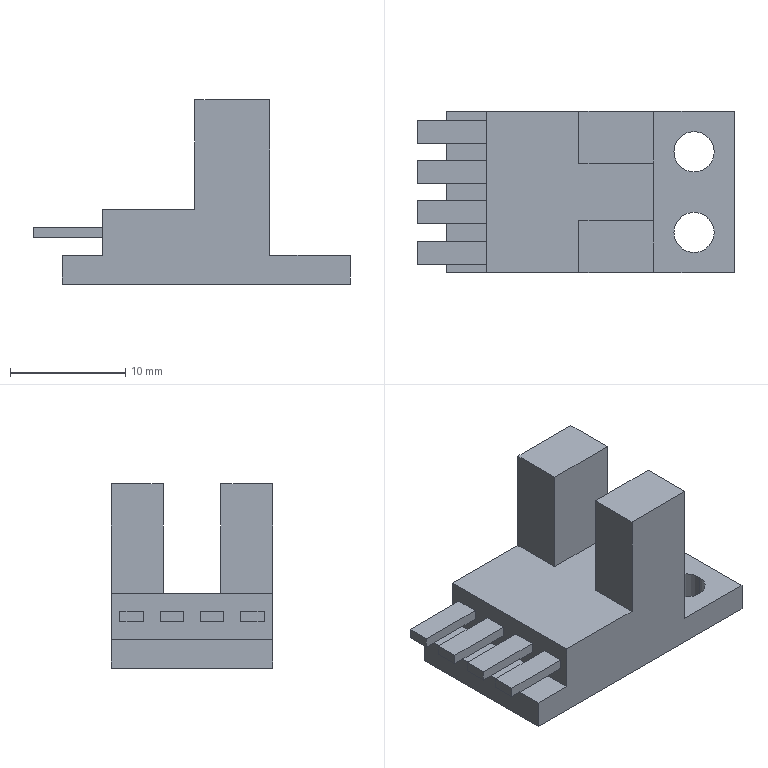Part | SolidWorks | features BaseBody 1 | 1 solid | 40 faces | box 27.5 x 14 x 16 mm | volume 2237 mm3 | plane 36 | cylinder 4 | commonest cylinder face diameters 3.5 x4
STEP:
#1=CARTESIAN_POINT('',(23.25,-10.5,0.));
#2=VERTEX_POINT('',#1);
#3=CARTESIAN_POINT('',(19.75,-10.5,0.));
#4=VERTEX_POINT('',#3);
#5=CARTESIAN_POINT('',(21.5,-10.5,0.));
#6=DIRECTION('',(0.,0.,-1.));
#7=DIRECTION('',(1.,0.,0.));
#8=AXIS2_PLACEMENT_3D('',#5,#6,#7);
#9=CIRCLE('',#8,1.75);
#10=EDGE_CURVE('',#2,#4,#9,.T.);
#11=ORIENTED_EDGE('',*,*,#10,.T.);
#12=CARTESIAN_POINT('',(19.75,-10.5,2.5));
#13=VERTEX_POINT('',#12);
#14=CARTESIAN_POINT('',(19.75,-10.5,-7.));
#15=DIRECTION('',(0.,0.,1.));
#16=VECTOR('',#15,1000.);
#17=LINE('',#14,#16);
#18=EDGE_CURVE('',#4,#13,#17,.T.);
#19=ORIENTED_EDGE('',*,*,#18,.T.);
#20=CARTESIAN_POINT('',(23.25,-10.5,2.5));
#21=VERTEX_POINT('',#20);
#22=CARTESIAN_POINT('',(21.5,-10.5,2.5));
#23=DIRECTION('',(0.,0.,-1.));
#24=DIRECTION('',(1.,0.,0.));
#25=AXIS2_PLACEMENT_3D('',#22,#23,#24);
#26=CIRCLE('',#25,1.75);
#27=EDGE_CURVE('',#21,#13,#26,.T.);
#28=ORIENTED_EDGE('',*,*,#27,.F.);
#29=CARTESIAN_POINT('',(23.25,-10.5,-7.));
#30=DIRECTION('',(0.,0.,1.));
#31=VECTOR('',#30,1000.);
#32=LINE('',#29,#31);
#33=EDGE_CURVE('',#2,#21,#32,.T.);
#34=ORIENTED_EDGE('',*,*,#33,.F.);
#35=EDGE_LOOP('',(#11,#19,#28,#34));
#36=FACE_OUTER_BOUND('',#35,.T.);
#37=CARTESIAN_POINT('',(21.5,-10.5,-7.));
#38=DIRECTION('',(0.,0.,1.));
#39=DIRECTION('',(1.,0.,0.));
#40=AXIS2_PLACEMENT_3D('',#37,#38,#39);
#41=CYLINDRICAL_SURFACE('',#40,1.75);
#42=ADVANCED_FACE('',(#36),#41,.F.);
#43=CARTESIAN_POINT('',(23.25,-3.5,0.));
#44=VERTEX_POINT('',#43);
#45=CARTESIAN_POINT('',(19.75,-3.5,0.));
#46=VERTEX_POINT('',#45);
#47=CARTESIAN_POINT('',(21.5,-3.5,0.));
#48=DIRECTION('',(0.,0.,-1.));
#49=DIRECTION('',(1.,0.,0.));
#50=AXIS2_PLACEMENT_3D('',#47,#48,#49);
#51=CIRCLE('',#50,1.75);
#52=EDGE_CURVE('',#44,#46,#51,.T.);
#53=ORIENTED_EDGE('',*,*,#52,.T.);
#54=CARTESIAN_POINT('',(19.75,-3.5,2.5));
#55=VERTEX_POINT('',#54);
#56=CARTESIAN_POINT('',(19.75,-3.5,-7.));
#57=DIRECTION('',(0.,0.,1.));
#58=VECTOR('',#57,1000.);
#59=LINE('',#56,#58);
#60=EDGE_CURVE('',#46,#55,#59,.T.);
#61=ORIENTED_EDGE('',*,*,#60,.T.);
#62=CARTESIAN_POINT('',(23.25,-3.5,2.5));
#63=VERTEX_POINT('',#62);
#64=CARTESIAN_POINT('',(21.5,-3.5,2.5));
#65=DIRECTION('',(0.,0.,-1.));
#66=DIRECTION('',(1.,0.,0.));
#67=AXIS2_PLACEMENT_3D('',#64,#65,#66);
#68=CIRCLE('',#67,1.75);
#69=EDGE_CURVE('',#63,#55,#68,.T.);
#70=ORIENTED_EDGE('',*,*,#69,.F.);
#71=CARTESIAN_POINT('',(23.25,-3.5,-7.));
#72=DIRECTION('',(0.,0.,1.));
#73=VECTOR('',#72,1000.);
#74=LINE('',#71,#73);
#75=EDGE_CURVE('',#44,#63,#74,.T.);
#76=ORIENTED_EDGE('',*,*,#75,.F.);
#77=EDGE_LOOP('',(#53,#61,#70,#76));
#78=FACE_OUTER_BOUND('',#77,.T.);
#79=CARTESIAN_POINT('',(21.5,-3.5,-7.));
#80=DIRECTION('',(0.,0.,1.));
#81=DIRECTION('',(1.,0.,0.));
#82=AXIS2_PLACEMENT_3D('',#79,#80,#81);
#83=CYLINDRICAL_SURFACE('',#82,1.75);
#84=ADVANCED_FACE('',(#78),#83,.F.);
#85=ORIENTED_EDGE('',*,*,#10,.F.);
#86=CARTESIAN_POINT('',(21.5,-10.5,0.));
#87=DIRECTION('',(0.,0.,-1.));
#88=DIRECTION('',(1.,0.,0.));
#89=AXIS2_PLACEMENT_3D('',#86,#87,#88);
#90=CIRCLE('',#89,1.75);
#91=EDGE_CURVE('',#4,#2,#90,.T.);
#92=ORIENTED_EDGE('',*,*,#91,.F.);
#93=EDGE_LOOP('',(#85,#92));
#94=FACE_BOUND('',#93,.T.);
#95=ORIENTED_EDGE('',*,*,#52,.F.);
#96=CARTESIAN_POINT('',(21.5,-3.5,0.));
#97=DIRECTION('',(0.,0.,-1.));
#98=DIRECTION('',(1.,0.,0.));
#99=AXIS2_PLACEMENT_3D('',#96,#97,#98);
#100=CIRCLE('',#99,1.75);
#101=EDGE_CURVE('',#46,#44,#100,.T.);
#102=ORIENTED_EDGE('',*,*,#101,.F.);
#103=EDGE_LOOP('',(#95,#102));
#104=FACE_BOUND('',#103,.T.);
#105=CARTESIAN_POINT('',(0.,0.,0.));
#106=VERTEX_POINT('',#105);
#107=CARTESIAN_POINT('',(0.,-14.,0.));
#108=VERTEX_POINT('',#107);
#109=CARTESIAN_POINT('',(0.,0.,0.));
#110=DIRECTION('',(0.,-1.,0.));
#111=VECTOR('',#110,1000.);
#112=LINE('',#109,#111);
#113=EDGE_CURVE('',#106,#108,#112,.T.);
#114=ORIENTED_EDGE('',*,*,#113,.F.);
#115=CARTESIAN_POINT('',(25.,0.,0.));
#116=VERTEX_POINT('',#115);
#117=CARTESIAN_POINT('',(0.,0.,0.));
#118=DIRECTION('',(-1.,0.,0.));
#119=VECTOR('',#118,1000.);
#120=LINE('',#117,#119);
#121=EDGE_CURVE('',#116,#106,#120,.T.);
#122=ORIENTED_EDGE('',*,*,#121,.F.);
#123=CARTESIAN_POINT('',(25.,-14.,0.));
#124=VERTEX_POINT('',#123);
#125=CARTESIAN_POINT('',(25.,0.,0.));
#126=DIRECTION('',(0.,1.,0.));
#127=VECTOR('',#126,1000.);
#128=LINE('',#125,#127);
#129=EDGE_CURVE('',#124,#116,#128,.T.);
#130=ORIENTED_EDGE('',*,*,#129,.F.);
#131=CARTESIAN_POINT('',(0.,-14.,0.));
#132=DIRECTION('',(1.,0.,0.));
#133=VECTOR('',#132,1000.);
#134=LINE('',#131,#133);
#135=EDGE_CURVE('',#108,#124,#134,.T.);
#136=ORIENTED_EDGE('',*,*,#135,.F.);
#137=EDGE_LOOP('',(#114,#122,#130,#136));
#138=FACE_OUTER_BOUND('',#137,.T.);
#139=CARTESIAN_POINT('',(0.,0.,0.));
#140=DIRECTION('',(0.,0.,1.));
#141=DIRECTION('',(1.,0.,0.));
#142=AXIS2_PLACEMENT_3D('',#139,#140,#141);
#143=PLANE('',#142);
#144=ADVANCED_FACE('',(#94,#104,#138),#143,.F.);
#145=ORIENTED_EDGE('',*,*,#18,.F.);
#146=ORIENTED_EDGE('',*,*,#91,.T.);
#147=ORIENTED_EDGE('',*,*,#33,.T.);
#148=CARTESIAN_POINT('',(21.5,-10.5,2.5));
#149=DIRECTION('',(0.,0.,-1.));
#150=DIRECTION('',(1.,0.,0.));
#151=AXIS2_PLACEMENT_3D('',#148,#149,#150);
#152=CIRCLE('',#151,1.75);
#153=EDGE_CURVE('',#13,#21,#152,.T.);
#154=ORIENTED_EDGE('',*,*,#153,.F.);
#155=EDGE_LOOP('',(#145,#146,#147,#154));
#156=FACE_OUTER_BOUND('',#155,.T.);
#157=CARTESIAN_POINT('',(21.5,-10.5,-7.));
#158=DIRECTION('',(0.,0.,1.));
#159=DIRECTION('',(1.,0.,0.));
#160=AXIS2_PLACEMENT_3D('',#157,#158,#159);
#161=CYLINDRICAL_SURFACE('',#160,1.75);
#162=ADVANCED_FACE('',(#156),#161,.F.);
#163=ORIENTED_EDGE('',*,*,#60,.F.);
#164=ORIENTED_EDGE('',*,*,#101,.T.);
#165=ORIENTED_EDGE('',*,*,#75,.T.);
#166=CARTESIAN_POINT('',(21.5,-3.5,2.5));
#167=DIRECTION('',(0.,0.,-1.));
#168=DIRECTION('',(1.,0.,0.));
#169=AXIS2_PLACEMENT_3D('',#166,#167,#168);
#170=CIRCLE('',#169,1.75);
#171=EDGE_CURVE('',#55,#63,#170,.T.);
#172=ORIENTED_EDGE('',*,*,#171,.F.);
#173=EDGE_LOOP('',(#163,#164,#165,#172));
#174=FACE_OUTER_BOUND('',#173,.T.);
#175=CARTESIAN_POINT('',(21.5,-3.5,-7.));
#176=DIRECTION('',(0.,0.,1.));
#177=DIRECTION('',(1.,0.,0.));
#178=AXIS2_PLACEMENT_3D('',#175,#176,#177);
#179=CYLINDRICAL_SURFACE('',#178,1.75);
#180=ADVANCED_FACE('',(#174),#179,.F.);
#181=CARTESIAN_POINT('',(0.,-14.,2.5));
#182=VERTEX_POINT('',#181);
#183=CARTESIAN_POINT('',(3.5,-14.,2.5));
#184=VERTEX_POINT('',#183);
#185=CARTESIAN_POINT('',(0.,-14.,2.5));
#186=DIRECTION('',(1.,0.,0.));
#187=VECTOR('',#186,1000.);
#188=LINE('',#185,#187);
#189=EDGE_CURVE('',#182,#184,#188,.T.);
#190=ORIENTED_EDGE('',*,*,#189,.F.);
#191=CARTESIAN_POINT('',(0.,-14.,2.5));
#192=DIRECTION('',(0.,0.,1.));
#193=VECTOR('',#192,1000.);
#194=LINE('',#191,#193);
#195=EDGE_CURVE('',#108,#182,#194,.T.);
#196=ORIENTED_EDGE('',*,*,#195,.F.);
#197=ORIENTED_EDGE('',*,*,#135,.T.);
#198=CARTESIAN_POINT('',(25.,-14.,2.5));
#199=VERTEX_POINT('',#198);
#200=CARTESIAN_POINT('',(25.,-14.,2.5));
#201=DIRECTION('',(0.,0.,-1.));
#202=VECTOR('',#201,1000.);
#203=LINE('',#200,#202);
#204=EDGE_CURVE('',#199,#124,#203,.T.);
#205=ORIENTED_EDGE('',*,*,#204,.F.);
#206=CARTESIAN_POINT('',(18.,-14.,2.5));
#207=VERTEX_POINT('',#206);
#208=CARTESIAN_POINT('',(0.,-14.,2.5));
#209=DIRECTION('',(1.,0.,0.));
#210=VECTOR('',#209,1000.);
#211=LINE('',#208,#210);
#212=EDGE_CURVE('',#207,#199,#211,.T.);
#213=ORIENTED_EDGE('',*,*,#212,.F.);
#214=CARTESIAN_POINT('',(18.,-14.,16.));
#215=VERTEX_POINT('',#214);
#216=CARTESIAN_POINT('',(18.,-14.,2.5));
#217=DIRECTION('',(0.,0.,-1.));
#218=VECTOR('',#217,1000.);
#219=LINE('',#216,#218);
#220=EDGE_CURVE('',#215,#207,#219,.T.);
#221=ORIENTED_EDGE('',*,*,#220,.F.);
#222=CARTESIAN_POINT('',(11.5,-14.,16.));
#223=VERTEX_POINT('',#222);
#224=CARTESIAN_POINT('',(0.,-14.,16.));
#225=DIRECTION('',(1.,0.,0.));
#226=VECTOR('',#225,1000.);
#227=LINE('',#224,#226);
#228=EDGE_CURVE('',#223,#215,#227,.T.);
#229=ORIENTED_EDGE('',*,*,#228,.F.);
#230=CARTESIAN_POINT('',(11.5,-14.,6.5));
#231=VERTEX_POINT('',#230);
#232=CARTESIAN_POINT('',(11.5,-14.,2.5));
#233=DIRECTION('',(0.,0.,1.));
#234=VECTOR('',#233,1000.);
#235=LINE('',#232,#234);
#236=EDGE_CURVE('',#231,#223,#235,.T.);
#237=ORIENTED_EDGE('',*,*,#236,.F.);
#238=CARTESIAN_POINT('',(3.5,-14.,6.5));
#239=VERTEX_POINT('',#238);
#240=CARTESIAN_POINT('',(0.,-14.,6.5));
#241=DIRECTION('',(1.,0.,0.));
#242=VECTOR('',#241,1000.);
#243=LINE('',#240,#242);
#244=EDGE_CURVE('',#239,#231,#243,.T.);
#245=ORIENTED_EDGE('',*,*,#244,.F.);
#246=CARTESIAN_POINT('',(3.5,-14.,2.5));
#247=DIRECTION('',(0.,0.,1.));
#248=VECTOR('',#247,1000.);
#249=LINE('',#246,#248);
#250=EDGE_CURVE('',#184,#239,#249,.T.);
#251=ORIENTED_EDGE('',*,*,#250,.F.);
#252=EDGE_LOOP('',(#190,#196,#197,#205,#213,#221,#229,#237,#245,#251));
#253=FACE_OUTER_BOUND('',#252,.T.);
#254=CARTESIAN_POINT('',(0.,-14.,2.5));
#255=DIRECTION('',(0.,1.,0.));
#256=DIRECTION('',(-1.,0.,0.));
#257=AXIS2_PLACEMENT_3D('',#254,#255,#256);
#258=PLANE('',#257);
#259=ADVANCED_FACE('',(#253),#258,.F.);
#260=ORIENTED_EDGE('',*,*,#113,.T.);
#261=ORIENTED_EDGE('',*,*,#195,.T.);
#262=CARTESIAN_POINT('',(0.,0.,2.5));
#263=VERTEX_POINT('',#262);
#264=CARTESIAN_POINT('',(0.,0.,2.5));
#265=DIRECTION('',(0.,-1.,0.));
#266=VECTOR('',#265,1000.);
#267=LINE('',#264,#266);
#268=EDGE_CURVE('',#263,#182,#267,.T.);
#269=ORIENTED_EDGE('',*,*,#268,.F.);
#270=CARTESIAN_POINT('',(0.,0.,2.5));
#271=DIRECTION('',(0.,0.,1.));
#272=VECTOR('',#271,1000.);
#273=LINE('',#270,#272);
#274=EDGE_CURVE('',#106,#263,#273,.T.);
#275=ORIENTED_EDGE('',*,*,#274,.F.);
#276=EDGE_LOOP('',(#260,#261,#269,#275));
#277=FACE_OUTER_BOUND('',#276,.T.);
#278=CARTESIAN_POINT('',(0.,0.,2.5));
#279=DIRECTION('',(1.,0.,0.));
#280=DIRECTION('',(0.,1.,0.));
#281=AXIS2_PLACEMENT_3D('',#278,#279,#280);
#282=PLANE('',#281);
#283=ADVANCED_FACE('',(#277),#282,.F.);
#284=CARTESIAN_POINT('',(25.,0.,2.5));
#285=VERTEX_POINT('',#284);
#286=CARTESIAN_POINT('',(18.,0.,2.5));
#287=VERTEX_POINT('',#286);
#288=CARTESIAN_POINT('',(0.,0.,2.5));
#289=DIRECTION('',(-1.,0.,0.));
#290=VECTOR('',#289,1000.);
#291=LINE('',#288,#290);
#292=EDGE_CURVE('',#285,#287,#291,.T.);
#293=ORIENTED_EDGE('',*,*,#292,.F.);
#294=CARTESIAN_POINT('',(25.,0.,2.5));
#295=DIRECTION('',(0.,0.,1.));
#296=VECTOR('',#295,1000.);
#297=LINE('',#294,#296);
#298=EDGE_CURVE('',#116,#285,#297,.T.);
#299=ORIENTED_EDGE('',*,*,#298,.F.);
#300=ORIENTED_EDGE('',*,*,#121,.T.);
#301=ORIENTED_EDGE('',*,*,#274,.T.);
#302=CARTESIAN_POINT('',(3.5,0.,2.5));
#303=VERTEX_POINT('',#302);
#304=CARTESIAN_POINT('',(0.,0.,2.5));
#305=DIRECTION('',(-1.,0.,0.));
#306=VECTOR('',#305,1000.);
#307=LINE('',#304,#306);
#308=EDGE_CURVE('',#303,#263,#307,.T.);
#309=ORIENTED_EDGE('',*,*,#308,.F.);
#310=CARTESIAN_POINT('',(3.5,0.,6.5));
#311=VERTEX_POINT('',#310);
#312=CARTESIAN_POINT('',(3.5,0.,2.5));
#313=DIRECTION('',(0.,0.,-1.));
#314=VECTOR('',#313,1000.);
#315=LINE('',#312,#314);
#316=EDGE_CURVE('',#311,#303,#315,.T.);
#317=ORIENTED_EDGE('',*,*,#316,.F.);
#318=CARTESIAN_POINT('',(11.5,0.,6.5));
#319=VERTEX_POINT('',#318);
#320=CARTESIAN_POINT('',(0.,0.,6.5));
#321=DIRECTION('',(-1.,0.,0.));
#322=VECTOR('',#321,1000.);
#323=LINE('',#320,#322);
#324=EDGE_CURVE('',#319,#311,#323,.T.);
#325=ORIENTED_EDGE('',*,*,#324,.F.);
#326=CARTESIAN_POINT('',(11.5,0.,16.));
#327=VERTEX_POINT('',#326);
#328=CARTESIAN_POINT('',(11.5,0.,2.5));
#329=DIRECTION('',(0.,0.,-1.));
#330=VECTOR('',#329,1000.);
#331=LINE('',#328,#330);
#332=EDGE_CURVE('',#327,#319,#331,.T.);
#333=ORIENTED_EDGE('',*,*,#332,.F.);
#334=CARTESIAN_POINT('',(18.,0.,16.));
#335=VERTEX_POINT('',#334);
#336=CARTESIAN_POINT('',(0.,0.,16.));
#337=DIRECTION('',(-1.,0.,0.));
#338=VECTOR('',#337,1000.);
#339=LINE('',#336,#338);
#340=EDGE_CURVE('',#335,#327,#339,.T.);
#341=ORIENTED_EDGE('',*,*,#340,.F.);
#342=CARTESIAN_POINT('',(18.,0.,2.5));
#343=DIRECTION('',(0.,0.,1.));
#344=VECTOR('',#343,1000.);
#345=LINE('',#342,#344);
#346=EDGE_CURVE('',#287,#335,#345,.T.);
#347=ORIENTED_EDGE('',*,*,#346,.F.);
#348=EDGE_LOOP('',(#293,#299,#300,#301,#309,#317,#325,#333,#341,#347));
#349=FACE_OUTER_BOUND('',#348,.T.);
#350=CARTESIAN_POINT('',(0.,0.,2.5));
#351=DIRECTION('',(0.,-1.,0.));
#352=DIRECTION('',(0.,0.,-1.));
#353=AXIS2_PLACEMENT_3D('',#350,#351,#352);
#354=PLANE('',#353);
#355=ADVANCED_FACE('',(#349),#354,.F.);
#356=ORIENTED_EDGE('',*,*,#129,.T.);
#357=ORIENTED_EDGE('',*,*,#298,.T.);
#358=CARTESIAN_POINT('',(25.,0.,2.5));
#359=DIRECTION('',(0.,1.,0.));
#360=VECTOR('',#359,1000.);
#361=LINE('',#358,#360);
#362=EDGE_CURVE('',#199,#285,#361,.T.);
#363=ORIENTED_EDGE('',*,*,#362,.F.);
#364=ORIENTED_EDGE('',*,*,#204,.T.);
#365=EDGE_LOOP('',(#356,#357,#363,#364));
#366=FACE_OUTER_BOUND('',#365,.T.);
#367=CARTESIAN_POINT('',(25.,0.,2.5));
#368=DIRECTION('',(-1.,0.,0.));
#369=DIRECTION('',(0.,0.,1.));
#370=AXIS2_PLACEMENT_3D('',#367,#368,#369);
#371=PLANE('',#370);
#372=ADVANCED_FACE('',(#366),#371,.F.);
#373=ORIENTED_EDGE('',*,*,#27,.T.);
#374=ORIENTED_EDGE('',*,*,#153,.T.);
#375=EDGE_LOOP('',(#373,#374));
#376=FACE_BOUND('',#375,.T.);
#377=ORIENTED_EDGE('',*,*,#69,.T.);
#378=ORIENTED_EDGE('',*,*,#171,.T.);
#379=EDGE_LOOP('',(#377,#378));
#380=FACE_BOUND('',#379,.T.);
#381=CARTESIAN_POINT('',(18.,0.,2.5));
#382=DIRECTION('',(0.,-1.,0.));
#383=VECTOR('',#382,1000.);
#384=LINE('',#381,#383);
#385=EDGE_CURVE('',#287,#207,#384,.T.);
#386=ORIENTED_EDGE('',*,*,#385,.T.);
#387=ORIENTED_EDGE('',*,*,#212,.T.);
#388=ORIENTED_EDGE('',*,*,#362,.T.);
#389=ORIENTED_EDGE('',*,*,#292,.T.);
#390=EDGE_LOOP('',(#386,#387,#388,#389));
#391=FACE_OUTER_BOUND('',#390,.T.);
#392=CARTESIAN_POINT('',(0.,0.,2.5));
#393=DIRECTION('',(0.,0.,1.));
#394=DIRECTION('',(1.,0.,0.));
#395=AXIS2_PLACEMENT_3D('',#392,#393,#394);
#396=PLANE('',#395);
#397=ADVANCED_FACE('',(#376,#380,#391),#396,.T.);
#398=CARTESIAN_POINT('',(3.5,-9.75,4.946));
#399=VERTEX_POINT('',#398);
#400=CARTESIAN_POINT('',(3.5,-7.75,4.946));
#401=VERTEX_POINT('',#400);
#402=CARTESIAN_POINT('',(3.5,0.,4.946));
#403=DIRECTION('',(0.,1.,0.));
#404=VECTOR('',#403,1000.);
#405=LINE('',#402,#404);
#406=EDGE_CURVE('',#399,#401,#405,.T.);
#407=ORIENTED_EDGE('',*,*,#406,.F.);
#408=CARTESIAN_POINT('',(3.5,-9.75,4.054));
#409=VERTEX_POINT('',#408);
#410=CARTESIAN_POINT('',(3.5,-9.75,4.054));
#411=DIRECTION('',(0.,0.,-1.));
#412=VECTOR('',#411,1000.);
#413=LINE('',#410,#412);
#414=EDGE_CURVE('',#399,#409,#413,.T.);
#415=ORIENTED_EDGE('',*,*,#414,.T.);
#416=CARTESIAN_POINT('',(3.5,-7.75,4.054));
#417=VERTEX_POINT('',#416);
#418=CARTESIAN_POINT('',(3.5,0.,4.054));
#419=DIRECTION('',(0.,-1.,0.));
#420=VECTOR('',#419,1000.);
#421=LINE('',#418,#420);
#422=EDGE_CURVE('',#417,#409,#421,.T.);
#423=ORIENTED_EDGE('',*,*,#422,.F.);
#424=CARTESIAN_POINT('',(3.5,-7.75,4.054));
#425=DIRECTION('',(0.,0.,1.));
#426=VECTOR('',#425,1000.);
#427=LINE('',#424,#426);
#428=EDGE_CURVE('',#417,#401,#427,.T.);
#429=ORIENTED_EDGE('',*,*,#428,.T.);
#430=EDGE_LOOP('',(#407,#415,#423,#429));
#431=FACE_BOUND('',#430,.T.);
#432=CARTESIAN_POINT('',(3.5,-2.75,4.946));
#433=VERTEX_POINT('',#432);
#434=CARTESIAN_POINT('',(3.5,-0.75,4.946));
#435=VERTEX_POINT('',#434);
#436=CARTESIAN_POINT('',(3.5,0.,4.946));
#437=DIRECTION('',(0.,1.,0.));
#438=VECTOR('',#437,1000.);
#439=LINE('',#436,#438);
#440=EDGE_CURVE('',#433,#435,#439,.T.);
#441=ORIENTED_EDGE('',*,*,#440,.F.);
#442=CARTESIAN_POINT('',(3.5,-2.75,4.054));
#443=VERTEX_POINT('',#442);
#444=CARTESIAN_POINT('',(3.5,-2.75,4.054));
#445=DIRECTION('',(0.,0.,-1.));
#446=VECTOR('',#445,1000.);
#447=LINE('',#444,#446);
#448=EDGE_CURVE('',#433,#443,#447,.T.);
#449=ORIENTED_EDGE('',*,*,#448,.T.);
#450=CARTESIAN_POINT('',(3.5,-0.75,4.054));
#451=VERTEX_POINT('',#450);
#452=CARTESIAN_POINT('',(3.5,0.,4.054));
#453=DIRECTION('',(0.,-1.,0.));
#454=VECTOR('',#453,1000.);
#455=LINE('',#452,#454);
#456=EDGE_CURVE('',#451,#443,#455,.T.);
#457=ORIENTED_EDGE('',*,*,#456,.F.);
#458=CARTESIAN_POINT('',(3.5,-0.75,4.054));
#459=DIRECTION('',(0.,0.,1.));
#460=VECTOR('',#459,1000.);
#461=LINE('',#458,#460);
#462=EDGE_CURVE('',#451,#435,#461,.T.);
#463=ORIENTED_EDGE('',*,*,#462,.T.);
#464=EDGE_LOOP('',(#441,#449,#457,#463));
#465=FACE_BOUND('',#464,.T.);
#466=CARTESIAN_POINT('',(3.5,0.,6.5));
#467=DIRECTION('',(0.,-1.,0.));
#468=VECTOR('',#467,1000.);
#469=LINE('',#466,#468);
#470=EDGE_CURVE('',#311,#239,#469,.T.);
#471=ORIENTED_EDGE('',*,*,#470,.F.);
#472=ORIENTED_EDGE('',*,*,#316,.T.);
#473=CARTESIAN_POINT('',(3.5,0.,2.5));
#474=DIRECTION('',(0.,1.,0.));
#475=VECTOR('',#474,1000.);
#476=LINE('',#473,#475);
#477=EDGE_CURVE('',#184,#303,#476,.T.);
#478=ORIENTED_EDGE('',*,*,#477,.F.);
#479=ORIENTED_EDGE('',*,*,#250,.T.);
#480=EDGE_LOOP('',(#471,#472,#478,#479));
#481=FACE_OUTER_BOUND('',#480,.T.);
#482=CARTESIAN_POINT('',(3.5,-6.25,4.946));
#483=VERTEX_POINT('',#482);
#484=CARTESIAN_POINT('',(3.5,-4.25,4.946));
#485=VERTEX_POINT('',#484);
#486=CARTESIAN_POINT('',(3.5,0.,4.946));
#487=DIRECTION('',(0.,1.,0.));
#488=VECTOR('',#487,1000.);
#489=LINE('',#486,#488);
#490=EDGE_CURVE('',#483,#485,#489,.T.);
#491=ORIENTED_EDGE('',*,*,#490,.F.);
#492=CARTESIAN_POINT('',(3.5,-6.25,4.054));
#493=VERTEX_POINT('',#492);
#494=CARTESIAN_POINT('',(3.5,-6.25,4.054));
#495=DIRECTION('',(0.,0.,-1.));
#496=VECTOR('',#495,1000.);
#497=LINE('',#494,#496);
#498=EDGE_CURVE('',#483,#493,#497,.T.);
#499=ORIENTED_EDGE('',*,*,#498,.T.);
#500=CARTESIAN_POINT('',(3.5,-4.25,4.054));
#501=VERTEX_POINT('',#500);
#502=CARTESIAN_POINT('',(3.5,0.,4.054));
#503=DIRECTION('',(0.,-1.,0.));
#504=VECTOR('',#503,1000.);
#505=LINE('',#502,#504);
#506=EDGE_CURVE('',#501,#493,#505,.T.);
#507=ORIENTED_EDGE('',*,*,#506,.F.);
#508=CARTESIAN_POINT('',(3.5,-4.25,4.054));
#509=DIRECTION('',(0.,0.,1.));
#510=VECTOR('',#509,1000.);
#511=LINE('',#508,#510);
#512=EDGE_CURVE('',#501,#485,#511,.T.);
#513=ORIENTED_EDGE('',*,*,#512,.T.);
#514=EDGE_LOOP('',(#491,#499,#507,#513));
#515=FACE_BOUND('',#514,.T.);
#516=CARTESIAN_POINT('',(3.5,-13.25,4.946));
#517=VERTEX_POINT('',#516);
#518=CARTESIAN_POINT('',(3.5,-11.25,4.946));
#519=VERTEX_POINT('',#518);
#520=CARTESIAN_POINT('',(3.5,0.,4.946));
#521=DIRECTION('',(0.,1.,0.));
#522=VECTOR('',#521,1000.);
#523=LINE('',#520,#522);
#524=EDGE_CURVE('',#517,#519,#523,.T.);
#525=ORIENTED_EDGE('',*,*,#524,.F.);
#526=CARTESIAN_POINT('',(3.5,-13.25,4.054));
#527=VERTEX_POINT('',#526);
#528=CARTESIAN_POINT('',(3.5,-13.25,4.054));
#529=DIRECTION('',(0.,0.,-1.));
#530=VECTOR('',#529,1000.);
#531=LINE('',#528,#530);
#532=EDGE_CURVE('',#517,#527,#531,.T.);
#533=ORIENTED_EDGE('',*,*,#532,.T.);
#534=CARTESIAN_POINT('',(3.5,-11.25,4.054));
#535=VERTEX_POINT('',#534);
#536=CARTESIAN_POINT('',(3.5,0.,4.054));
#537=DIRECTION('',(0.,-1.,0.));
#538=VECTOR('',#537,1000.);
#539=LINE('',#536,#538);
#540=EDGE_CURVE('',#535,#527,#539,.T.);
#541=ORIENTED_EDGE('',*,*,#540,.F.);
#542=CARTESIAN_POINT('',(3.5,-11.25,4.054));
#543=DIRECTION('',(0.,0.,1.));
#544=VECTOR('',#543,1000.);
#545=LINE('',#542,#544);
#546=EDGE_CURVE('',#535,#519,#545,.T.);
#547=ORIENTED_EDGE('',*,*,#546,.T.);
#548=EDGE_LOOP('',(#525,#533,#541,#547));
#549=FACE_BOUND('',#548,.T.);
#550=CARTESIAN_POINT('',(3.5,0.,16.));
#551=DIRECTION('',(1.,0.,0.));
#552=DIRECTION('',(0.,1.,0.));
#553=AXIS2_PLACEMENT_3D('',#550,#551,#552);
#554=PLANE('',#553);
#555=ADVANCED_FACE('',(#431,#465,#481,#515,#549),#554,.F.);
#556=ORIENTED_EDGE('',*,*,#477,.T.);
#557=ORIENTED_EDGE('',*,*,#308,.T.);
#558=ORIENTED_EDGE('',*,*,#268,.T.);
#559=ORIENTED_EDGE('',*,*,#189,.T.);
#560=EDGE_LOOP('',(#556,#557,#558,#559));
#561=FACE_OUTER_BOUND('',#560,.T.);
#562=CARTESIAN_POINT('',(0.,0.,2.5));
#563=DIRECTION('',(0.,0.,1.));
#564=DIRECTION('',(1.,0.,0.));
#565=AXIS2_PLACEMENT_3D('',#562,#563,#564);
#566=PLANE('',#565);
#567=ADVANCED_FACE('',(#561),#566,.T.);
#568=CARTESIAN_POINT('',(18.,-9.5,16.));
#569=VERTEX_POINT('',#568);
#570=CARTESIAN_POINT('',(18.,0.,16.));
#571=DIRECTION('',(0.,1.,0.));
#572=VECTOR('',#571,1000.);
#573=LINE('',#570,#572);
#574=EDGE_CURVE('',#215,#569,#573,.T.);
#575=ORIENTED_EDGE('',*,*,#574,.F.);
#576=ORIENTED_EDGE('',*,*,#220,.T.);
#577=ORIENTED_EDGE('',*,*,#385,.F.);
#578=ORIENTED_EDGE('',*,*,#346,.T.);
#579=CARTESIAN_POINT('',(18.,-4.5,16.));
#580=VERTEX_POINT('',#579);
#581=CARTESIAN_POINT('',(18.,0.,16.));
#582=DIRECTION('',(0.,1.,0.));
#583=VECTOR('',#582,1000.);
#584=LINE('',#581,#583);
#585=EDGE_CURVE('',#580,#335,#584,.T.);
#586=ORIENTED_EDGE('',*,*,#585,.F.);
#587=CARTESIAN_POINT('',(18.,-4.5,6.5));
#588=VERTEX_POINT('',#587);
#589=CARTESIAN_POINT('',(18.,-4.5,16.));
#590=DIRECTION('',(0.,0.,1.));
#591=VECTOR('',#590,1000.);
#592=LINE('',#589,#591);
#593=EDGE_CURVE('',#588,#580,#592,.T.);
#594=ORIENTED_EDGE('',*,*,#593,.F.);
#595=CARTESIAN_POINT('',(18.,-9.5,6.5));
#596=VERTEX_POINT('',#595);
#597=CARTESIAN_POINT('',(18.,0.,6.5));
#598=DIRECTION('',(0.,1.,0.));
#599=VECTOR('',#598,1000.);
#600=LINE('',#597,#599);
#601=EDGE_CURVE('',#596,#588,#600,.T.);
#602=ORIENTED_EDGE('',*,*,#601,.F.);
#603=CARTESIAN_POINT('',(18.,-9.5,16.));
#604=DIRECTION('',(0.,0.,-1.));
#605=VECTOR('',#604,1000.);
#606=LINE('',#603,#605);
#607=EDGE_CURVE('',#569,#596,#606,.T.);
#608=ORIENTED_EDGE('',*,*,#607,.F.);
#609=EDGE_LOOP('',(#575,#576,#577,#578,#586,#594,#602,#608));
#610=FACE_OUTER_BOUND('',#609,.T.);
#611=CARTESIAN_POINT('',(18.,0.,16.));
#612=DIRECTION('',(-1.,0.,0.));
#613=DIRECTION('',(0.,0.,1.));
#614=AXIS2_PLACEMENT_3D('',#611,#612,#613);
#615=PLANE('',#614);
#616=ADVANCED_FACE('',(#610),#615,.F.);
#617=ORIENTED_EDGE('',*,*,#574,.T.);
#618=CARTESIAN_POINT('',(11.5,-9.5,16.));
#619=VERTEX_POINT('',#618);
#620=CARTESIAN_POINT('',(0.,-9.5,16.));
#621=DIRECTION('',(1.,0.,0.));
#622=VECTOR('',#621,1000.);
#623=LINE('',#620,#622);
#624=EDGE_CURVE('',#619,#569,#623,.T.);
#625=ORIENTED_EDGE('',*,*,#624,.F.);
#626=CARTESIAN_POINT('',(11.5,0.,16.));
#627=DIRECTION('',(0.,1.,0.));
#628=VECTOR('',#627,1000.);
#629=LINE('',#626,#628);
#630=EDGE_CURVE('',#223,#619,#629,.T.);
#631=ORIENTED_EDGE('',*,*,#630,.F.);
#632=ORIENTED_EDGE('',*,*,#228,.T.);
#633=EDGE_LOOP('',(#617,#625,#631,#632));
#634=FACE_OUTER_BOUND('',#633,.T.);
#635=CARTESIAN_POINT('',(0.,0.,16.));
#636=DIRECTION('',(0.,0.,-1.));
#637=DIRECTION('',(-1.,0.,0.));
#638=AXIS2_PLACEMENT_3D('',#635,#636,#637);
#639=PLANE('',#638);
#640=ADVANCED_FACE('',(#634),#639,.F.);
#641=ORIENTED_EDGE('',*,*,#630,.T.);
#642=CARTESIAN_POINT('',(11.5,-9.5,6.5));
#643=VERTEX_POINT('',#642);
#644=CARTESIAN_POINT('',(11.5,-9.5,6.5));
#645=DIRECTION('',(0.,0.,1.));
#646=VECTOR('',#645,1000.);
#647=LINE('',#644,#646);
#648=EDGE_CURVE('',#643,#619,#647,.T.);
#649=ORIENTED_EDGE('',*,*,#648,.F.);
#650=CARTESIAN_POINT('',(11.5,0.,6.5));
#651=DIRECTION('',(0.,1.,0.));
#652=VECTOR('',#651,1000.);
#653=LINE('',#650,#652);
#654=EDGE_CURVE('',#231,#643,#653,.T.);
#655=ORIENTED_EDGE('',*,*,#654,.F.);
#656=ORIENTED_EDGE('',*,*,#236,.T.);
#657=EDGE_LOOP('',(#641,#649,#655,#656));
#658=FACE_OUTER_BOUND('',#657,.T.);
#659=CARTESIAN_POINT('',(11.5,0.,6.5));
#660=DIRECTION('',(1.,0.,0.));
#661=DIRECTION('',(0.,1.,0.));
#662=AXIS2_PLACEMENT_3D('',#659,#660,#661);
#663=PLANE('',#662);
#664=ADVANCED_FACE('',(#658),#663,.F.);
#665=ORIENTED_EDGE('',*,*,#470,.T.);
#666=ORIENTED_EDGE('',*,*,#244,.T.);
#667=ORIENTED_EDGE('',*,*,#654,.T.);
#668=CARTESIAN_POINT('',(0.,-9.5,6.5));
#669=DIRECTION('',(1.,0.,0.));
#670=VECTOR('',#669,1000.);
#671=LINE('',#668,#670);
#672=EDGE_CURVE('',#643,#596,#671,.T.);
#673=ORIENTED_EDGE('',*,*,#672,.T.);
#674=ORIENTED_EDGE('',*,*,#601,.T.);
#675=CARTESIAN_POINT('',(11.5,-4.5,6.5));
#676=VERTEX_POINT('',#675);
#677=CARTESIAN_POINT('',(0.,-4.5,6.5));
#678=DIRECTION('',(-1.,0.,0.));
#679=VECTOR('',#678,1000.);
#680=LINE('',#677,#679);
#681=EDGE_CURVE('',#588,#676,#680,.T.);
#682=ORIENTED_EDGE('',*,*,#681,.T.);
#683=CARTESIAN_POINT('',(11.5,0.,6.5));
#684=DIRECTION('',(0.,1.,0.));
#685=VECTOR('',#684,1000.);
#686=LINE('',#683,#685);
#687=EDGE_CURVE('',#676,#319,#686,.T.);
#688=ORIENTED_EDGE('',*,*,#687,.T.);
#689=ORIENTED_EDGE('',*,*,#324,.T.);
#690=EDGE_LOOP('',(#665,#666,#667,#673,#674,#682,#688,#689));
#691=FACE_OUTER_BOUND('',#690,.T.);
#692=CARTESIAN_POINT('',(0.,0.,6.5));
#693=DIRECTION('',(0.,0.,1.));
#694=DIRECTION('',(1.,0.,0.));
#695=AXIS2_PLACEMENT_3D('',#692,#693,#694);
#696=PLANE('',#695);
#697=ADVANCED_FACE('',(#691),#696,.T.);
#698=ORIENTED_EDGE('',*,*,#687,.F.);
#699=CARTESIAN_POINT('',(11.5,-4.5,16.));
#700=VERTEX_POINT('',#699);
#701=CARTESIAN_POINT('',(11.5,-4.5,6.5));
#702=DIRECTION('',(0.,0.,-1.));
#703=VECTOR('',#702,1000.);
#704=LINE('',#701,#703);
#705=EDGE_CURVE('',#700,#676,#704,.T.);
#706=ORIENTED_EDGE('',*,*,#705,.F.);
#707=CARTESIAN_POINT('',(11.5,0.,16.));
#708=DIRECTION('',(0.,-1.,0.));
#709=VECTOR('',#708,1000.);
#710=LINE('',#707,#709);
#711=EDGE_CURVE('',#327,#700,#710,.T.);
#712=ORIENTED_EDGE('',*,*,#711,.F.);
#713=ORIENTED_EDGE('',*,*,#332,.T.);
#714=EDGE_LOOP('',(#698,#706,#712,#713));
#715=FACE_OUTER_BOUND('',#714,.T.);
#716=CARTESIAN_POINT('',(11.5,0.,6.5));
#717=DIRECTION('',(1.,0.,0.));
#718=DIRECTION('',(0.,1.,0.));
#719=AXIS2_PLACEMENT_3D('',#716,#717,#718);
#720=PLANE('',#719);
#721=ADVANCED_FACE('',(#715),#720,.F.);
#722=ORIENTED_EDGE('',*,*,#711,.T.);
#723=CARTESIAN_POINT('',(0.,-4.5,16.));
#724=DIRECTION('',(-1.,0.,0.));
#725=VECTOR('',#724,1000.);
#726=LINE('',#723,#725);
#727=EDGE_CURVE('',#580,#700,#726,.T.);
#728=ORIENTED_EDGE('',*,*,#727,.F.);
#729=ORIENTED_EDGE('',*,*,#585,.T.);
#730=ORIENTED_EDGE('',*,*,#340,.T.);
#731=EDGE_LOOP('',(#722,#728,#729,#730));
#732=FACE_OUTER_BOUND('',#731,.T.);
#733=CARTESIAN_POINT('',(0.,0.,16.));
#734=DIRECTION('',(0.,0.,-1.));
#735=DIRECTION('',(-1.,0.,0.));
#736=AXIS2_PLACEMENT_3D('',#733,#734,#735);
#737=PLANE('',#736);
#738=ADVANCED_FACE('',(#732),#737,.F.);
#739=ORIENTED_EDGE('',*,*,#406,.T.);
#740=CARTESIAN_POINT('',(-2.5,-7.75,4.946));
#741=VERTEX_POINT('',#740);
#742=CARTESIAN_POINT('',(-2.5,-7.75,4.946));
#743=DIRECTION('',(1.,0.,0.));
#744=VECTOR('',#743,1000.);
#745=LINE('',#742,#744);
#746=EDGE_CURVE('',#741,#401,#745,.T.);
#747=ORIENTED_EDGE('',*,*,#746,.F.);
#748=CARTESIAN_POINT('',(-2.5,-9.75,4.946));
#749=VERTEX_POINT('',#748);
#750=CARTESIAN_POINT('',(-2.5,-7.75,4.946));
#751=DIRECTION('',(0.,1.,0.));
#752=VECTOR('',#751,1000.);
#753=LINE('',#750,#752);
#754=EDGE_CURVE('',#749,#741,#753,.T.);
#755=ORIENTED_EDGE('',*,*,#754,.F.);
#756=CARTESIAN_POINT('',(-2.5,-9.75,4.946));
#757=DIRECTION('',(-1.,0.,0.));
#758=VECTOR('',#757,1000.);
#759=LINE('',#756,#758);
#760=EDGE_CURVE('',#399,#749,#759,.T.);
#761=ORIENTED_EDGE('',*,*,#760,.F.);
#762=EDGE_LOOP('',(#739,#747,#755,#761));
#763=FACE_OUTER_BOUND('',#762,.T.);
#764=CARTESIAN_POINT('',(-2.5,-7.75,4.946));
#765=DIRECTION('',(0.,0.,-1.));
#766=DIRECTION('',(0.,1.,0.));
#767=AXIS2_PLACEMENT_3D('',#764,#765,#766);
#768=PLANE('',#767);
#769=ADVANCED_FACE('',(#763),#768,.F.);
#770=ORIENTED_EDGE('',*,*,#422,.T.);
#771=CARTESIAN_POINT('',(-2.5,-9.75,4.054));
#772=VERTEX_POINT('',#771);
#773=CARTESIAN_POINT('',(-2.5,-9.75,4.054));
#774=DIRECTION('',(1.,0.,0.));
#775=VECTOR('',#774,1000.);
#776=LINE('',#773,#775);
#777=EDGE_CURVE('',#772,#409,#776,.T.);
#778=ORIENTED_EDGE('',*,*,#777,.F.);
#779=CARTESIAN_POINT('',(-2.5,-7.75,4.054));
#780=VERTEX_POINT('',#779);
#781=CARTESIAN_POINT('',(-2.5,-7.75,4.054));
#782=DIRECTION('',(0.,-1.,0.));
#783=VECTOR('',#782,1000.);
#784=LINE('',#781,#783);
#785=EDGE_CURVE('',#780,#772,#784,.T.);
#786=ORIENTED_EDGE('',*,*,#785,.F.);
#787=CARTESIAN_POINT('',(-2.5,-7.75,4.054));
#788=DIRECTION('',(-1.,0.,0.));
#789=VECTOR('',#788,1000.);
#790=LINE('',#787,#789);
#791=EDGE_CURVE('',#417,#780,#790,.T.);
#792=ORIENTED_EDGE('',*,*,#791,.F.);
#793=EDGE_LOOP('',(#770,#778,#786,#792));
#794=FACE_OUTER_BOUND('',#793,.T.);
#795=CARTESIAN_POINT('',(-2.5,-7.75,4.054));
#796=DIRECTION('',(0.,0.,1.));
#797=DIRECTION('',(1.,0.,0.));
#798=AXIS2_PLACEMENT_3D('',#795,#796,#797);
#799=PLANE('',#798);
#800=ADVANCED_FACE('',(#794),#799,.F.);
#801=ORIENTED_EDGE('',*,*,#440,.T.);
#802=CARTESIAN_POINT('',(-2.5,-0.75,4.946));
#803=VERTEX_POINT('',#802);
#804=CARTESIAN_POINT('',(-2.5,-0.75,4.946));
#805=DIRECTION('',(1.,0.,0.));
#806=VECTOR('',#805,1000.);
#807=LINE('',#804,#806);
#808=EDGE_CURVE('',#803,#435,#807,.T.);
#809=ORIENTED_EDGE('',*,*,#808,.F.);
#810=CARTESIAN_POINT('',(-2.5,-2.75,4.946));
#811=VERTEX_POINT('',#810);
#812=CARTESIAN_POINT('',(-2.5,-0.75,4.946));
#813=DIRECTION('',(0.,1.,0.));
#814=VECTOR('',#813,1000.);
#815=LINE('',#812,#814);
#816=EDGE_CURVE('',#811,#803,#815,.T.);
#817=ORIENTED_EDGE('',*,*,#816,.F.);
#818=CARTESIAN_POINT('',(-2.5,-2.75,4.946));
#819=DIRECTION('',(-1.,0.,0.));
#820=VECTOR('',#819,1000.);
#821=LINE('',#818,#820);
#822=EDGE_CURVE('',#433,#811,#821,.T.);
#823=ORIENTED_EDGE('',*,*,#822,.F.);
#824=EDGE_LOOP('',(#801,#809,#817,#823));
#825=FACE_OUTER_BOUND('',#824,.T.);
#826=CARTESIAN_POINT('',(-2.5,-0.75,4.946));
#827=DIRECTION('',(0.,0.,-1.));
#828=DIRECTION('',(0.,1.,0.));
#829=AXIS2_PLACEMENT_3D('',#826,#827,#828);
#830=PLANE('',#829);
#831=ADVANCED_FACE('',(#825),#830,.F.);
#832=ORIENTED_EDGE('',*,*,#456,.T.);
#833=CARTESIAN_POINT('',(-2.5,-2.75,4.054));
#834=VERTEX_POINT('',#833);
#835=CARTESIAN_POINT('',(-2.5,-2.75,4.054));
#836=DIRECTION('',(1.,0.,0.));
#837=VECTOR('',#836,1000.);
#838=LINE('',#835,#837);
#839=EDGE_CURVE('',#834,#443,#838,.T.);
#840=ORIENTED_EDGE('',*,*,#839,.F.);
#841=CARTESIAN_POINT('',(-2.5,-0.75,4.054));
#842=VERTEX_POINT('',#841);
#843=CARTESIAN_POINT('',(-2.5,-0.75,4.054));
#844=DIRECTION('',(0.,-1.,0.));
#845=VECTOR('',#844,1000.);
#846=LINE('',#843,#845);
#847=EDGE_CURVE('',#842,#834,#846,.T.);
#848=ORIENTED_EDGE('',*,*,#847,.F.);
#849=CARTESIAN_POINT('',(-2.5,-0.75,4.054));
#850=DIRECTION('',(-1.,0.,0.));
#851=VECTOR('',#850,1000.);
#852=LINE('',#849,#851);
#853=EDGE_CURVE('',#451,#842,#852,.T.);
#854=ORIENTED_EDGE('',*,*,#853,.F.);
#855=EDGE_LOOP('',(#832,#840,#848,#854));
#856=FACE_OUTER_BOUND('',#855,.T.);
#857=CARTESIAN_POINT('',(-2.5,-0.75,4.054));
#858=DIRECTION('',(0.,0.,1.));
#859=DIRECTION('',(0.,-1.,0.));
#860=AXIS2_PLACEMENT_3D('',#857,#858,#859);
#861=PLANE('',#860);
#862=ADVANCED_FACE('',(#856),#861,.F.);
#863=ORIENTED_EDGE('',*,*,#490,.T.);
#864=CARTESIAN_POINT('',(-2.5,-4.25,4.946));
#865=VERTEX_POINT('',#864);
#866=CARTESIAN_POINT('',(-2.5,-4.25,4.946));
#867=DIRECTION('',(1.,0.,0.));
#868=VECTOR('',#867,1000.);
#869=LINE('',#866,#868);
#870=EDGE_CURVE('',#865,#485,#869,.T.);
#871=ORIENTED_EDGE('',*,*,#870,.F.);
#872=CARTESIAN_POINT('',(-2.5,-6.25,4.946));
#873=VERTEX_POINT('',#872);
#874=CARTESIAN_POINT('',(-2.5,-4.25,4.946));
#875=DIRECTION('',(0.,1.,0.));
#876=VECTOR('',#875,1000.);
#877=LINE('',#874,#876);
#878=EDGE_CURVE('',#873,#865,#877,.T.);
#879=ORIENTED_EDGE('',*,*,#878,.F.);
#880=CARTESIAN_POINT('',(-2.5,-6.25,4.946));
#881=DIRECTION('',(-1.,0.,0.));
#882=VECTOR('',#881,1000.);
#883=LINE('',#880,#882);
#884=EDGE_CURVE('',#483,#873,#883,.T.);
#885=ORIENTED_EDGE('',*,*,#884,.F.);
#886=EDGE_LOOP('',(#863,#871,#879,#885));
#887=FACE_OUTER_BOUND('',#886,.T.);
#888=CARTESIAN_POINT('',(-2.5,-4.25,4.946));
#889=DIRECTION('',(0.,0.,-1.));
#890=DIRECTION('',(-1.,0.,0.));
#891=AXIS2_PLACEMENT_3D('',#888,#889,#890);
#892=PLANE('',#891);
#893=ADVANCED_FACE('',(#887),#892,.F.);
#894=ORIENTED_EDGE('',*,*,#506,.T.);
#895=CARTESIAN_POINT('',(-2.5,-6.25,4.054));
#896=VERTEX_POINT('',#895);
#897=CARTESIAN_POINT('',(-2.5,-6.25,4.054));
#898=DIRECTION('',(1.,0.,0.));
#899=VECTOR('',#898,1000.);
#900=LINE('',#897,#899);
#901=EDGE_CURVE('',#896,#493,#900,.T.);
#902=ORIENTED_EDGE('',*,*,#901,.F.);
#903=CARTESIAN_POINT('',(-2.5,-4.25,4.054));
#904=VERTEX_POINT('',#903);
#905=CARTESIAN_POINT('',(-2.5,-4.25,4.054));
#906=DIRECTION('',(0.,-1.,0.));
#907=VECTOR('',#906,1000.);
#908=LINE('',#905,#907);
#909=EDGE_CURVE('',#904,#896,#908,.T.);
#910=ORIENTED_EDGE('',*,*,#909,.F.);
#911=CARTESIAN_POINT('',(-2.5,-4.25,4.054));
#912=DIRECTION('',(-1.,0.,0.));
#913=VECTOR('',#912,1000.);
#914=LINE('',#911,#913);
#915=EDGE_CURVE('',#501,#904,#914,.T.);
#916=ORIENTED_EDGE('',*,*,#915,.F.);
#917=EDGE_LOOP('',(#894,#902,#910,#916));
#918=FACE_OUTER_BOUND('',#917,.T.);
#919=CARTESIAN_POINT('',(-2.5,-4.25,4.054));
#920=DIRECTION('',(0.,0.,1.));
#921=DIRECTION('',(0.,-1.,0.));
#922=AXIS2_PLACEMENT_3D('',#919,#920,#921);
#923=PLANE('',#922);
#924=ADVANCED_FACE('',(#918),#923,.F.);
#925=ORIENTED_EDGE('',*,*,#524,.T.);
#926=CARTESIAN_POINT('',(-2.5,-11.25,4.946));
#927=VERTEX_POINT('',#926);
#928=CARTESIAN_POINT('',(-2.5,-11.25,4.946));
#929=DIRECTION('',(1.,0.,0.));
#930=VECTOR('',#929,1000.);
#931=LINE('',#928,#930);
#932=EDGE_CURVE('',#927,#519,#931,.T.);
#933=ORIENTED_EDGE('',*,*,#932,.F.);
#934=CARTESIAN_POINT('',(-2.5,-13.25,4.946));
#935=VERTEX_POINT('',#934);
#936=CARTESIAN_POINT('',(-2.5,-11.25,4.946));
#937=DIRECTION('',(0.,1.,0.));
#938=VECTOR('',#937,1000.);
#939=LINE('',#936,#938);
#940=EDGE_CURVE('',#935,#927,#939,.T.);
#941=ORIENTED_EDGE('',*,*,#940,.F.);
#942=CARTESIAN_POINT('',(-2.5,-13.25,4.946));
#943=DIRECTION('',(-1.,0.,0.));
#944=VECTOR('',#943,1000.);
#945=LINE('',#942,#944);
#946=EDGE_CURVE('',#517,#935,#945,.T.);
#947=ORIENTED_EDGE('',*,*,#946,.F.);
#948=EDGE_LOOP('',(#925,#933,#941,#947));
#949=FACE_OUTER_BOUND('',#948,.T.);
#950=CARTESIAN_POINT('',(-2.5,-11.25,4.946));
#951=DIRECTION('',(0.,0.,-1.));
#952=DIRECTION('',(0.,1.,0.));
#953=AXIS2_PLACEMENT_3D('',#950,#951,#952);
#954=PLANE('',#953);
#955=ADVANCED_FACE('',(#949),#954,.F.);
#956=ORIENTED_EDGE('',*,*,#540,.T.);
#957=CARTESIAN_POINT('',(-2.5,-13.25,4.054));
#958=VERTEX_POINT('',#957);
#959=CARTESIAN_POINT('',(-2.5,-13.25,4.054));
#960=DIRECTION('',(1.,0.,0.));
#961=VECTOR('',#960,1000.);
#962=LINE('',#959,#961);
#963=EDGE_CURVE('',#958,#527,#962,.T.);
#964=ORIENTED_EDGE('',*,*,#963,.F.);
#965=CARTESIAN_POINT('',(-2.5,-11.25,4.054));
#966=VERTEX_POINT('',#965);
#967=CARTESIAN_POINT('',(-2.5,-11.25,4.054));
#968=DIRECTION('',(0.,-1.,0.));
#969=VECTOR('',#968,1000.);
#970=LINE('',#967,#969);
#971=EDGE_CURVE('',#966,#958,#970,.T.);
#972=ORIENTED_EDGE('',*,*,#971,.F.);
#973=CARTESIAN_POINT('',(-2.5,-11.25,4.054));
#974=DIRECTION('',(-1.,0.,0.));
#975=VECTOR('',#974,1000.);
#976=LINE('',#973,#975);
#977=EDGE_CURVE('',#535,#966,#976,.T.);
#978=ORIENTED_EDGE('',*,*,#977,.F.);
#979=EDGE_LOOP('',(#956,#964,#972,#978));
#980=FACE_OUTER_BOUND('',#979,.T.);
#981=CARTESIAN_POINT('',(-2.5,-11.25,4.054));
#982=DIRECTION('',(0.,0.,1.));
#983=DIRECTION('',(0.,-1.,0.));
#984=AXIS2_PLACEMENT_3D('',#981,#982,#983);
#985=PLANE('',#984);
#986=ADVANCED_FACE('',(#980),#985,.F.);
#987=ORIENTED_EDGE('',*,*,#672,.F.);
#988=ORIENTED_EDGE('',*,*,#648,.T.);
#989=ORIENTED_EDGE('',*,*,#624,.T.);
#990=ORIENTED_EDGE('',*,*,#607,.T.);
#991=EDGE_LOOP('',(#987,#988,#989,#990));
#992=FACE_OUTER_BOUND('',#991,.T.);
#993=CARTESIAN_POINT('',(21.,-9.5,25.5));
#994=DIRECTION('',(0.,-1.,0.));
#995=DIRECTION('',(1.,0.,0.));
#996=AXIS2_PLACEMENT_3D('',#993,#994,#995);
#997=PLANE('',#996);
#998=ADVANCED_FACE('',(#992),#997,.F.);
#999=ORIENTED_EDGE('',*,*,#727,.T.);
#1000=ORIENTED_EDGE('',*,*,#705,.T.);
#1001=ORIENTED_EDGE('',*,*,#681,.F.);
#1002=ORIENTED_EDGE('',*,*,#593,.T.);
#1003=EDGE_LOOP('',(#999,#1000,#1001,#1002));
#1004=FACE_OUTER_BOUND('',#1003,.T.);
#1005=CARTESIAN_POINT('',(21.,-4.5,25.5));
#1006=DIRECTION('',(0.,1.,0.));
#1007=DIRECTION('',(-1.,0.,0.));
#1008=AXIS2_PLACEMENT_3D('',#1005,#1006,#1007);
#1009=PLANE('',#1008);
#1010=ADVANCED_FACE('',(#1004),#1009,.F.);
#1011=ORIENTED_EDGE('',*,*,#414,.F.);
#1012=ORIENTED_EDGE('',*,*,#760,.T.);
#1013=CARTESIAN_POINT('',(-2.5,-9.75,4.054));
#1014=DIRECTION('',(0.,0.,1.));
#1015=VECTOR('',#1014,1000.);
#1016=LINE('',#1013,#1015);
#1017=EDGE_CURVE('',#772,#749,#1016,.T.);
#1018=ORIENTED_EDGE('',*,*,#1017,.F.);
#1019=ORIENTED_EDGE('',*,*,#777,.T.);
#1020=EDGE_LOOP('',(#1011,#1012,#1018,#1019));
#1021=FACE_OUTER_BOUND('',#1020,.T.);
#1022=CARTESIAN_POINT('',(-2.5,-9.75,4.054));
#1023=DIRECTION('',(0.,1.,0.));
#1024=DIRECTION('',(-1.,0.,0.));
#1025=AXIS2_PLACEMENT_3D('',#1022,#1023,#1024);
#1026=PLANE('',#1025);
#1027=ADVANCED_FACE('',(#1021),#1026,.F.);
#1028=ORIENTED_EDGE('',*,*,#428,.F.);
#1029=ORIENTED_EDGE('',*,*,#791,.T.);
#1030=CARTESIAN_POINT('',(-2.5,-7.75,4.054));
#1031=DIRECTION('',(0.,0.,-1.));
#1032=VECTOR('',#1031,1000.);
#1033=LINE('',#1030,#1032);
#1034=EDGE_CURVE('',#741,#780,#1033,.T.);
#1035=ORIENTED_EDGE('',*,*,#1034,.F.);
#1036=ORIENTED_EDGE('',*,*,#746,.T.);
#1037=EDGE_LOOP('',(#1028,#1029,#1035,#1036));
#1038=FACE_OUTER_BOUND('',#1037,.T.);
#1039=CARTESIAN_POINT('',(-2.5,-7.75,4.054));
#1040=DIRECTION('',(0.,-1.,0.));
#1041=DIRECTION('',(1.,0.,0.));
#1042=AXIS2_PLACEMENT_3D('',#1039,#1040,#1041);
#1043=PLANE('',#1042);
#1044=ADVANCED_FACE('',(#1038),#1043,.F.);
#1045=ORIENTED_EDGE('',*,*,#754,.T.);
#1046=ORIENTED_EDGE('',*,*,#1034,.T.);
#1047=ORIENTED_EDGE('',*,*,#785,.T.);
#1048=ORIENTED_EDGE('',*,*,#1017,.T.);
#1049=EDGE_LOOP('',(#1045,#1046,#1047,#1048));
#1050=FACE_OUTER_BOUND('',#1049,.T.);
#1051=CARTESIAN_POINT('',(-2.5,0.,0.));
#1052=DIRECTION('',(-1.,0.,0.));
#1053=DIRECTION('',(0.,-1.,0.));
#1054=AXIS2_PLACEMENT_3D('',#1051,#1052,#1053);
#1055=PLANE('',#1054);
#1056=ADVANCED_FACE('',(#1050),#1055,.T.);
#1057=ORIENTED_EDGE('',*,*,#448,.F.);
#1058=ORIENTED_EDGE('',*,*,#822,.T.);
#1059=CARTESIAN_POINT('',(-2.5,-2.75,4.054));
#1060=DIRECTION('',(0.,0.,1.));
#1061=VECTOR('',#1060,1000.);
#1062=LINE('',#1059,#1061);
#1063=EDGE_CURVE('',#834,#811,#1062,.T.);
#1064=ORIENTED_EDGE('',*,*,#1063,.F.);
#1065=ORIENTED_EDGE('',*,*,#839,.T.);
#1066=EDGE_LOOP('',(#1057,#1058,#1064,#1065));
#1067=FACE_OUTER_BOUND('',#1066,.T.);
#1068=CARTESIAN_POINT('',(-2.5,-2.75,4.054));
#1069=DIRECTION('',(0.,1.,0.));
#1070=DIRECTION('',(-1.,0.,0.));
#1071=AXIS2_PLACEMENT_3D('',#1068,#1069,#1070);
#1072=PLANE('',#1071);
#1073=ADVANCED_FACE('',(#1067),#1072,.F.);
#1074=ORIENTED_EDGE('',*,*,#462,.F.);
#1075=ORIENTED_EDGE('',*,*,#853,.T.);
#1076=CARTESIAN_POINT('',(-2.5,-0.75,4.054));
#1077=DIRECTION('',(0.,0.,-1.));
#1078=VECTOR('',#1077,1000.);
#1079=LINE('',#1076,#1078);
#1080=EDGE_CURVE('',#803,#842,#1079,.T.);
#1081=ORIENTED_EDGE('',*,*,#1080,.F.);
#1082=ORIENTED_EDGE('',*,*,#808,.T.);
#1083=EDGE_LOOP('',(#1074,#1075,#1081,#1082));
#1084=FACE_OUTER_BOUND('',#1083,.T.);
#1085=CARTESIAN_POINT('',(-2.5,-0.75,4.054));
#1086=DIRECTION('',(0.,-1.,0.));
#1087=DIRECTION('',(1.,0.,0.));
#1088=AXIS2_PLACEMENT_3D('',#1085,#1086,#1087);
#1089=PLANE('',#1088);
#1090=ADVANCED_FACE('',(#1084),#1089,.F.);
#1091=ORIENTED_EDGE('',*,*,#816,.T.);
#1092=ORIENTED_EDGE('',*,*,#1080,.T.);
#1093=ORIENTED_EDGE('',*,*,#847,.T.);
#1094=ORIENTED_EDGE('',*,*,#1063,.T.);
#1095=EDGE_LOOP('',(#1091,#1092,#1093,#1094));
#1096=FACE_OUTER_BOUND('',#1095,.T.);
#1097=CARTESIAN_POINT('',(-2.5,0.,0.));
#1098=DIRECTION('',(-1.,0.,0.));
#1099=DIRECTION('',(0.,-1.,0.));
#1100=AXIS2_PLACEMENT_3D('',#1097,#1098,#1099);
#1101=PLANE('',#1100);
#1102=ADVANCED_FACE('',(#1096),#1101,.T.);
#1103=ORIENTED_EDGE('',*,*,#498,.F.);
#1104=ORIENTED_EDGE('',*,*,#884,.T.);
#1105=CARTESIAN_POINT('',(-2.5,-6.25,4.054));
#1106=DIRECTION('',(0.,0.,1.));
#1107=VECTOR('',#1106,1000.);
#1108=LINE('',#1105,#1107);
#1109=EDGE_CURVE('',#896,#873,#1108,.T.);
#1110=ORIENTED_EDGE('',*,*,#1109,.F.);
#1111=ORIENTED_EDGE('',*,*,#901,.T.);
#1112=EDGE_LOOP('',(#1103,#1104,#1110,#1111));
#1113=FACE_OUTER_BOUND('',#1112,.T.);
#1114=CARTESIAN_POINT('',(-2.5,-6.25,4.054));
#1115=DIRECTION('',(0.,1.,0.));
#1116=DIRECTION('',(0.,0.,1.));
#1117=AXIS2_PLACEMENT_3D('',#1114,#1115,#1116);
#1118=PLANE('',#1117);
#1119=ADVANCED_FACE('',(#1113),#1118,.F.);
#1120=ORIENTED_EDGE('',*,*,#512,.F.);
#1121=ORIENTED_EDGE('',*,*,#915,.T.);
#1122=CARTESIAN_POINT('',(-2.5,-4.25,4.054));
#1123=DIRECTION('',(0.,0.,-1.));
#1124=VECTOR('',#1123,1000.);
#1125=LINE('',#1122,#1124);
#1126=EDGE_CURVE('',#865,#904,#1125,.T.);
#1127=ORIENTED_EDGE('',*,*,#1126,.F.);
#1128=ORIENTED_EDGE('',*,*,#870,.T.);
#1129=EDGE_LOOP('',(#1120,#1121,#1127,#1128));
#1130=FACE_OUTER_BOUND('',#1129,.T.);
#1131=CARTESIAN_POINT('',(-2.5,-4.25,4.054));
#1132=DIRECTION('',(0.,-1.,0.));
#1133=DIRECTION('',(1.,0.,0.));
#1134=AXIS2_PLACEMENT_3D('',#1131,#1132,#1133);
#1135=PLANE('',#1134);
#1136=ADVANCED_FACE('',(#1130),#1135,.F.);
#1137=ORIENTED_EDGE('',*,*,#878,.T.);
#1138=ORIENTED_EDGE('',*,*,#1126,.T.);
#1139=ORIENTED_EDGE('',*,*,#909,.T.);
#1140=ORIENTED_EDGE('',*,*,#1109,.T.);
#1141=EDGE_LOOP('',(#1137,#1138,#1139,#1140));
#1142=FACE_OUTER_BOUND('',#1141,.T.);
#1143=CARTESIAN_POINT('',(-2.5,0.,0.));
#1144=DIRECTION('',(-1.,0.,0.));
#1145=DIRECTION('',(0.,-1.,0.));
#1146=AXIS2_PLACEMENT_3D('',#1143,#1144,#1145);
#1147=PLANE('',#1146);
#1148=ADVANCED_FACE('',(#1142),#1147,.T.);
#1149=ORIENTED_EDGE('',*,*,#532,.F.);
#1150=ORIENTED_EDGE('',*,*,#946,.T.);
#1151=CARTESIAN_POINT('',(-2.5,-13.25,4.054));
#1152=DIRECTION('',(0.,0.,1.));
#1153=VECTOR('',#1152,1000.);
#1154=LINE('',#1151,#1153);
#1155=EDGE_CURVE('',#958,#935,#1154,.T.);
#1156=ORIENTED_EDGE('',*,*,#1155,.F.);
#1157=ORIENTED_EDGE('',*,*,#963,.T.);
#1158=EDGE_LOOP('',(#1149,#1150,#1156,#1157));
#1159=FACE_OUTER_BOUND('',#1158,.T.);
#1160=CARTESIAN_POINT('',(-2.5,-13.25,4.054));
#1161=DIRECTION('',(0.,1.,0.));
#1162=DIRECTION('',(0.,0.,1.));
#1163=AXIS2_PLACEMENT_3D('',#1160,#1161,#1162);
#1164=PLANE('',#1163);
#1165=ADVANCED_FACE('',(#1159),#1164,.F.);
#1166=ORIENTED_EDGE('',*,*,#546,.F.);
#1167=ORIENTED_EDGE('',*,*,#977,.T.);
#1168=CARTESIAN_POINT('',(-2.5,-11.25,4.054));
#1169=DIRECTION('',(0.,0.,-1.));
#1170=VECTOR('',#1169,1000.);
#1171=LINE('',#1168,#1170);
#1172=EDGE_CURVE('',#927,#966,#1171,.T.);
#1173=ORIENTED_EDGE('',*,*,#1172,.F.);
#1174=ORIENTED_EDGE('',*,*,#932,.T.);
#1175=EDGE_LOOP('',(#1166,#1167,#1173,#1174));
#1176=FACE_OUTER_BOUND('',#1175,.T.);
#1177=CARTESIAN_POINT('',(-2.5,-11.25,4.054));
#1178=DIRECTION('',(0.,-1.,0.));
#1179=DIRECTION('',(1.,0.,0.));
#1180=AXIS2_PLACEMENT_3D('',#1177,#1178,#1179);
#1181=PLANE('',#1180);
#1182=ADVANCED_FACE('',(#1176),#1181,.F.);
#1183=ORIENTED_EDGE('',*,*,#940,.T.);
#1184=ORIENTED_EDGE('',*,*,#1172,.T.);
#1185=ORIENTED_EDGE('',*,*,#971,.T.);
#1186=ORIENTED_EDGE('',*,*,#1155,.T.);
#1187=EDGE_LOOP('',(#1183,#1184,#1185,#1186));
#1188=FACE_OUTER_BOUND('',#1187,.T.);
#1189=CARTESIAN_POINT('',(-2.5,0.,0.));
#1190=DIRECTION('',(-1.,0.,0.));
#1191=DIRECTION('',(0.,-1.,0.));
#1192=AXIS2_PLACEMENT_3D('',#1189,#1190,#1191);
#1193=PLANE('',#1192);
#1194=ADVANCED_FACE('',(#1188),#1193,.T.);
#1195=CLOSED_SHELL('',(#42,#84,#144,#162,#180,#259,#283,#355,#372,#397,#555,#567,#616,#640,#664,#697,#721,#738,#769,#800,#831,#862,#893,#924,#955,#986,#998,#1010,#1027,#1044,#1056,#1073,#1090,#1102,#1119,#1136,#1148,#1165,#1182,#1194));
#1196=MANIFOLD_SOLID_BREP('',#1195);
#1197=CARTESIAN_POINT('',(0.,0.,0.));
#1198=DIRECTION('',(0.,0.,1.));
#1199=DIRECTION('',(1.,0.,0.));
#1200=AXIS2_PLACEMENT_3D('',#1197,#1198,#1199);
#1201=(LENGTH_UNIT()NAMED_UNIT(*)SI_UNIT(.MILLI.,.METRE.));
#1202=UNCERTAINTY_MEASURE_WITH_UNIT(LENGTH_MEASURE(0.00001),#1201,'','');
#1203=(NAMED_UNIT(*)PLANE_ANGLE_UNIT()SI_UNIT($,.RADIAN.));
#1204=(NAMED_UNIT(*)SI_UNIT($,.STERADIAN.)SOLID_ANGLE_UNIT());
#1205=(GEOMETRIC_REPRESENTATION_CONTEXT(3)GLOBAL_UNCERTAINTY_ASSIGNED_CONTEXT((#1202))GLOBAL_UNIT_ASSIGNED_CONTEXT((#1201,#1203,#1204))REPRESENTATION_CONTEXT('',''));
#1206=ADVANCED_BREP_SHAPE_REPRESENTATION('',(#1196,#1200),#1205);